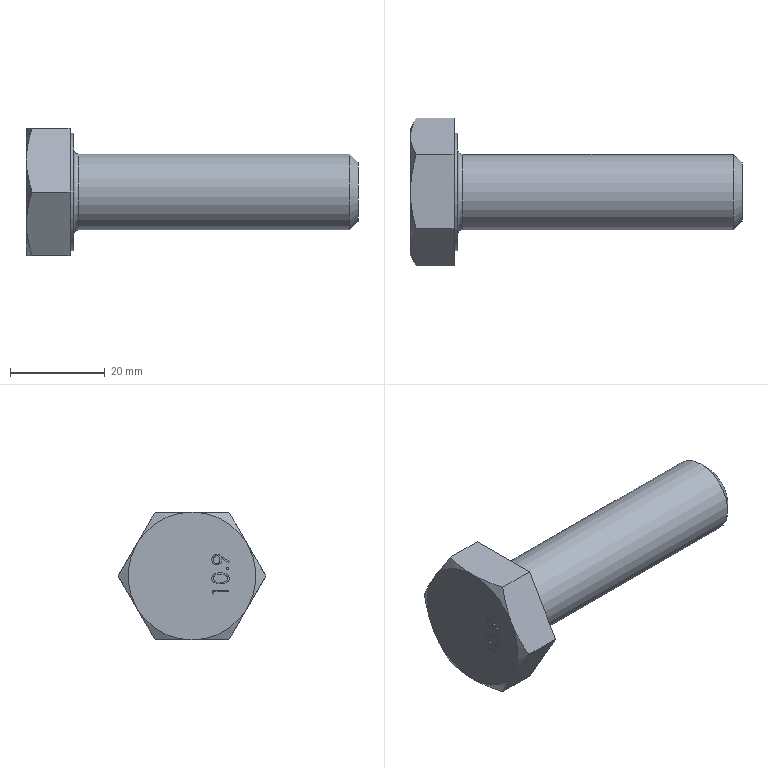Part | STEP file | Hex head bolt for steel structures M16×60 10.9 GBT1228-2006_M16×55 | 1 solid | 57 faces | box 70.1 x 31.177 x 27 mm | volume 18177 mm3 | plane 25 | spline 22 | cone 7 | cylinder 2 | torus 1 | commonest cylinder face diameters 16 x1 24.9 x1